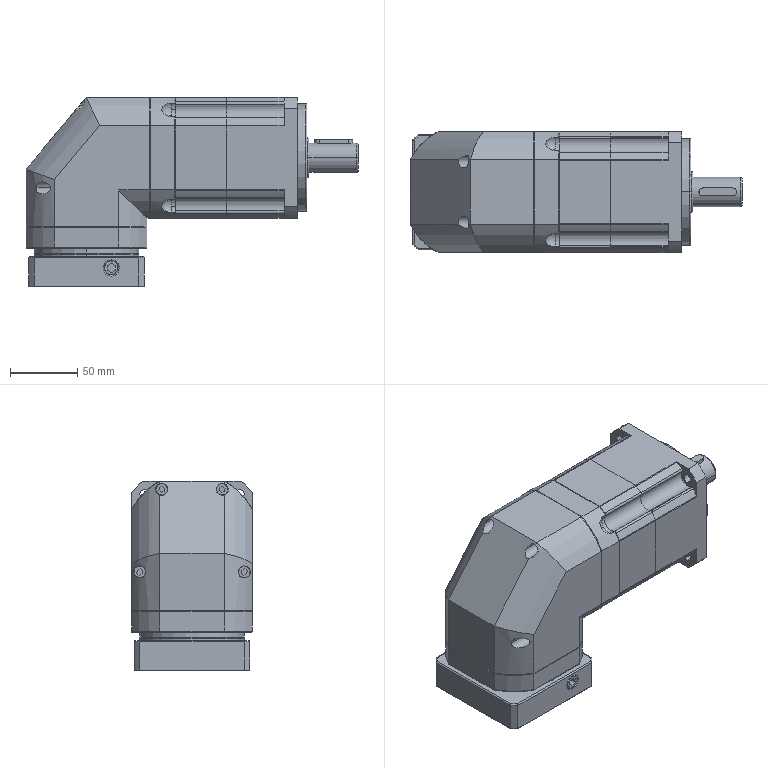Part | SolidWorks | features BaseBody 30 | 30 solids | 787 faces | box 247 x 90 x 141 mm | volume 1704334 mm3 | plane 321 | cylinder 291 | cone 93 | torus 71 | sphere 8 | spline 3 | commonest cylinder face diameters 3 x36 102 x34 8.5 x32 9 x29 14 x21 5.5 x16